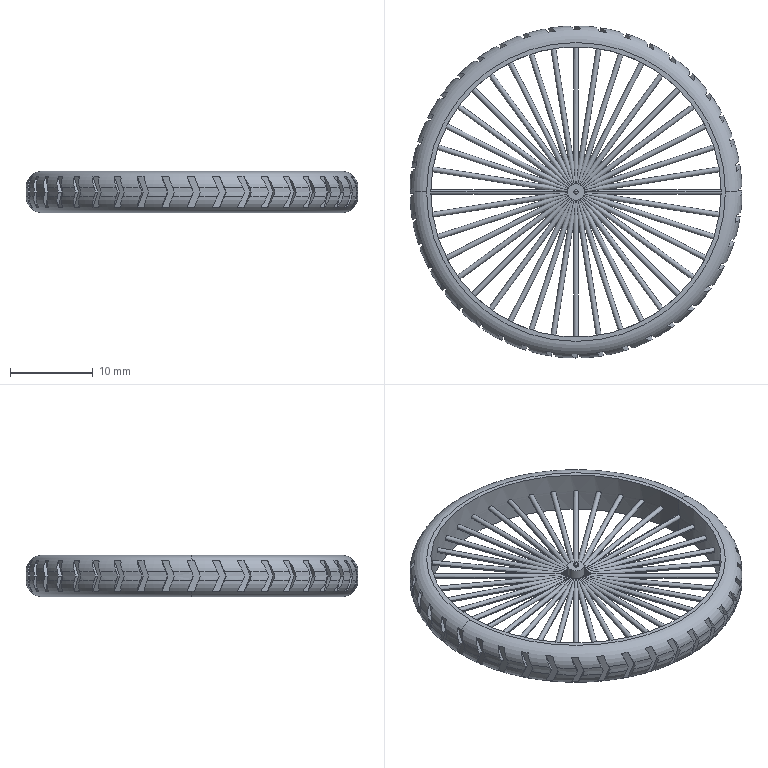Part | SolidWorks | features ICE 4, CirPattern 2, Fillet 2, Extrusion 1 | 1 solid | 339 faces | box 40 x 40 x 5 mm | volume 1401 mm3 | plane 204 | cylinder 129 | torus 4 | sphere 2 | commonest cylinder face diameters 0.6 x80 40 x41 2 x4 0.5 x2 35 x2